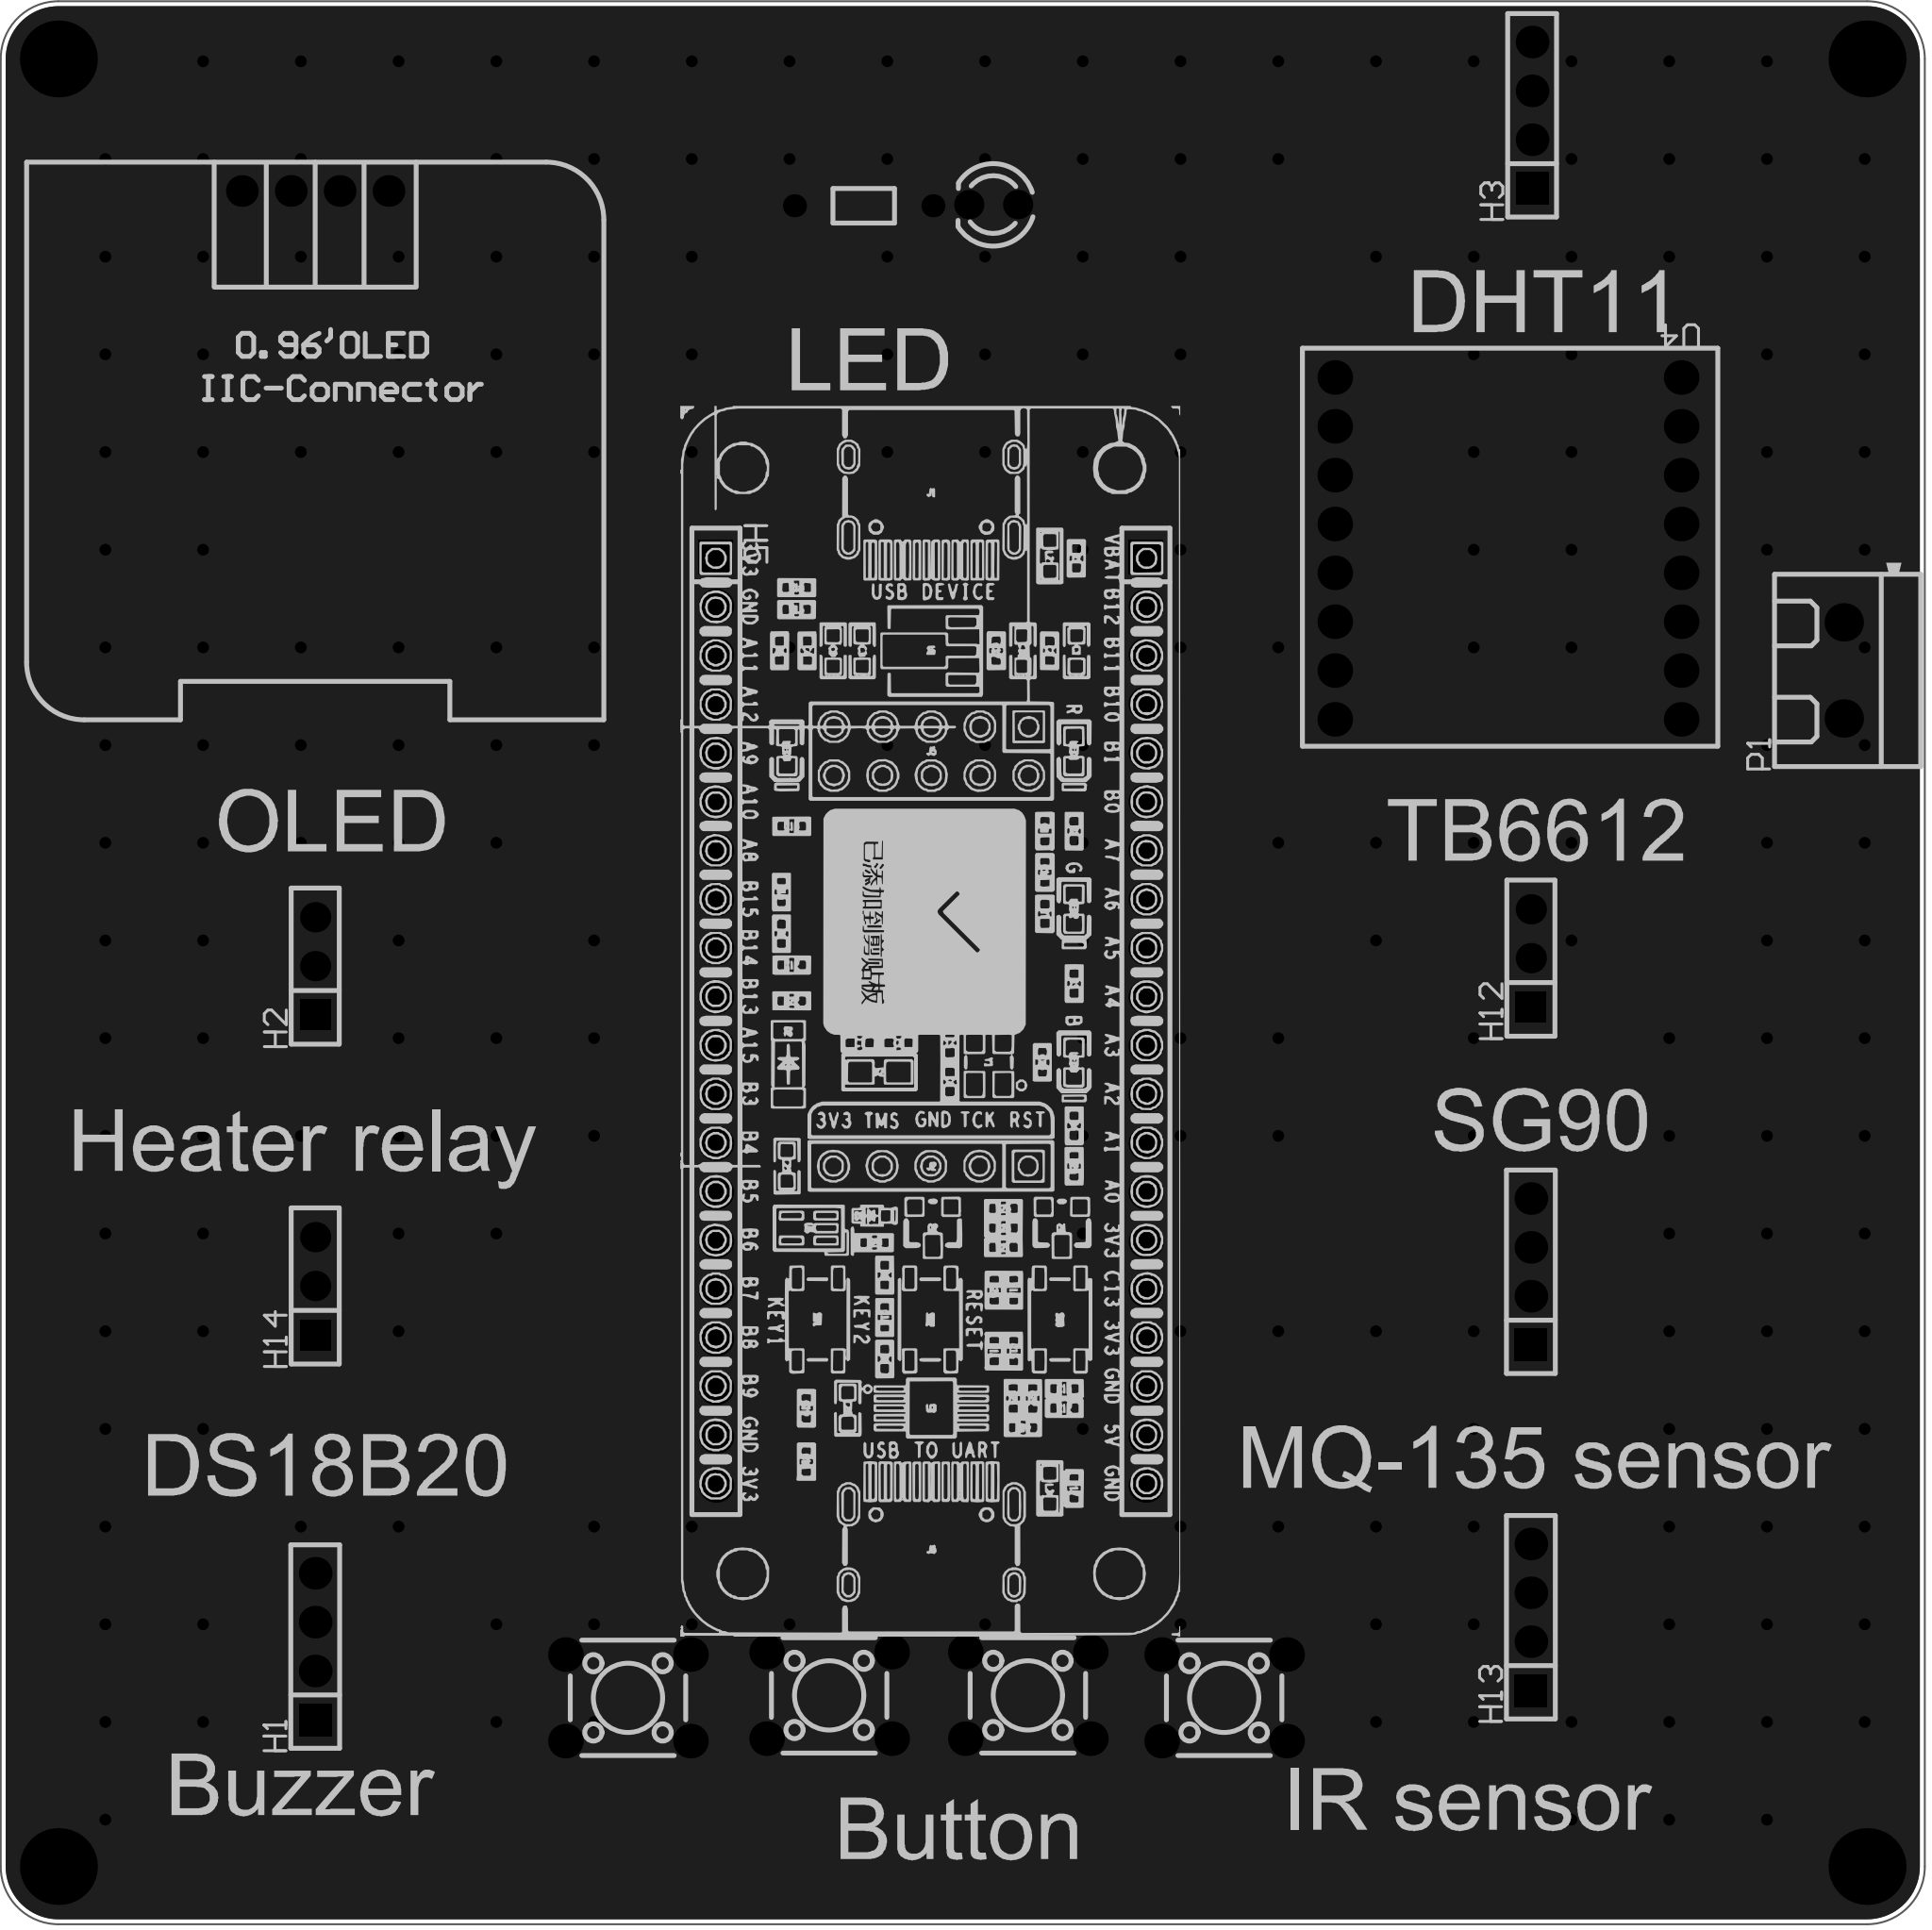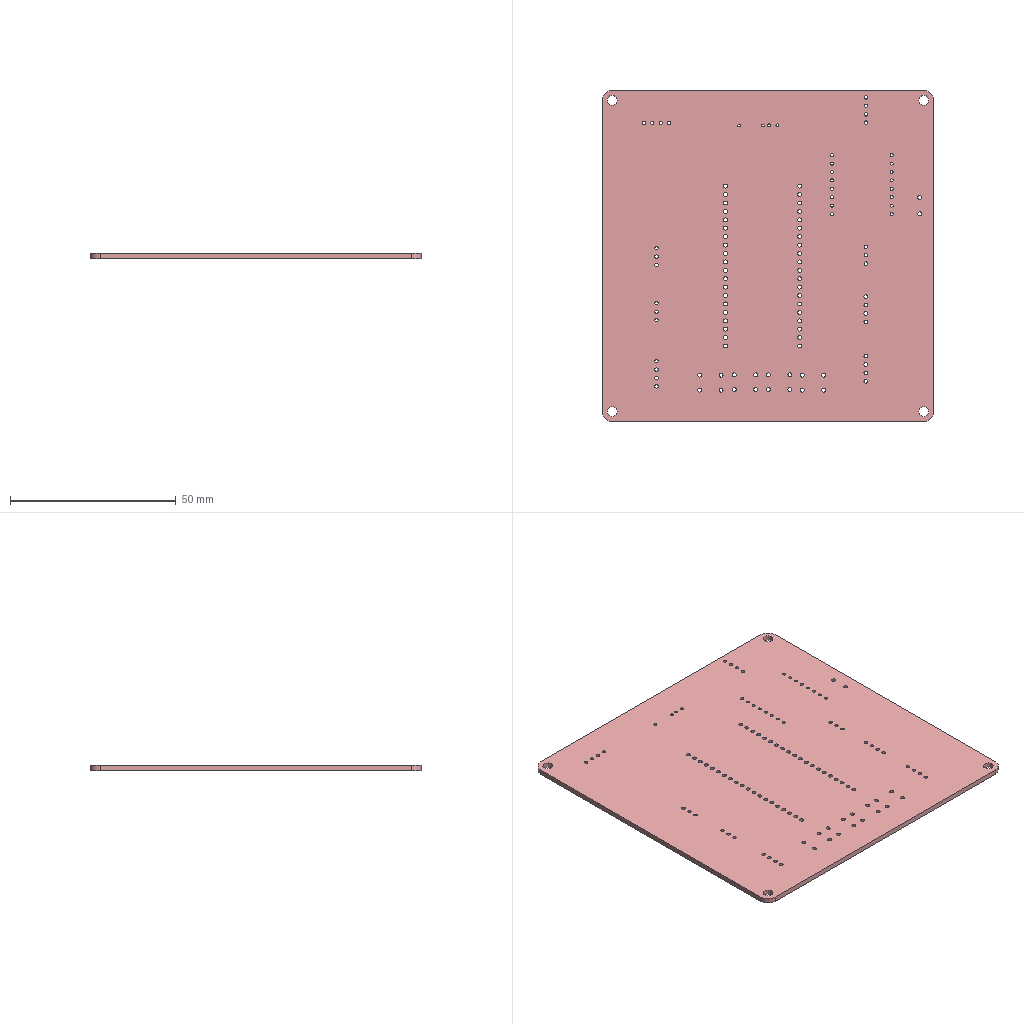Circuit board layout | Altium Designer | box 100 x 100 x 1.6 mm
Layer stack:
# Altium Designer layer stack of  (unit mm; dielectric type: 0 none, 1 core, 2 prepreg, 3 surface material)
index,name,kind,layer,copper_thickness_mm,dielectric_type,dielectric_thickness_mm,dielectric_material,dielectric_constant
0,Top Paste Mask Layer,other,,,,,,
1,Top Silkscreen Layer,other,,,,,,
2,Top Solder Mask Layer,dielectric,,,3,0.01,,3.3
3,Top Layer,copper,Top Layer,0.035,,,,
4,Dielectric1,dielectric,,,3,1.51,FR4,4.5
5,Bottom Layer,copper,Bottom Layer,0.035,,,,
6,Bottom Solder Mask Layer,dielectric,,,3,0.01,,3.3
7,Bottom Silkscreen Layer,other,,,,,,
8,Bottom Paste Mask Layer,other,,,,,,
# drill layer pairs: low layer,high layer
drill_pair,Top Layer,Bottom Layer
Part placement:
Designator,Comment,Layer,Footprint,Center-X(mm),Center-Y(mm),Rotation
SW1,,TopLayer,SW-TH_4P-L6.0-W6.0-P4.50-LS6.5,154.936,92.71,180
SW2,,TopLayer,SW-TH_4P-L6.0-W6.0-P4.50-LS6.5,134.407,92.837,180
SW3,,TopLayer,SW-TH_4P-L6.0-W6.0-P4.50-LS6.5,144.735,92.837,180
SW4,,TopLayer,SW-TH_4P-L6.0-W6.0-P4.50-LS6.5,123.952,92.71,180
H4,,TopLayer,HDR-TH_4P-P2.54-V-F,170.879,114.866,90
H6,,TopLayer,HDR-TH_20P-P2.54-V-F,150.869,127.888,270
LED1,,TopLayer,LED_TH-3mm,142.935,170.363,180
R1,220Ω,TopLayer,Res_1/8W,136.204,170.301,180
H2,,TopLayer,HDR-TH_3P-P2.54-V-F,107.696,130.762,90
OLED1,,TopLayer,0.96OLED_4P,107.696,171.069,0
H12,,TopLayer,HDR-TH_3P-P2.54-V-F,170.879,131.176,90
H13,,TopLayer,HDR-TH_4P-P2.54-V-F,170.879,96.902,90
H14,,TopLayer,HDR-TH_3P-P2.54-V-F,107.696,114.128,90
P1,KF301-2P terminal block,TopLayer,CONN-TH_XY301V-A-5.0-2P,187.141,146.139,90
U4,,TopLayer,tb6612,169.689,152.482,180
H1,,TopLayer,HDR-TH_4P-P2.54-V-F,107.696,95.377,90
H3,,TopLayer,HDR-TH_4P-P2.54-V-F,170.942,175.006,90
H5,,TopLayer,HDR-TH_20P-P2.54-V-F,128.524,127.889,270
Pad and via stacks:
# Altium Designer via and pad stacks of  (unit mm). Each distinct definition once, with the count of objects using it.
# via: kind,start_layer,end_layer,hole_mm,diameter_mm,mode(0 simple;1 top-mid-bottom;2 full stack),diameter_per_layer,count,example_net
# pad: kind,layer,hole_mm,hole_type(0 round;1 square;2 slot),plating,top_size,top_shape(1 round;2 rect;3 octagon;9 rounded rect),mid_size,bottom_size,mode,footprint,size_per_layer,count,example
pad,Multi-Layer,3,0,plated,4x4,1,4x4,4x4,0,,,4,1
pad,Multi-Layer,1.2,0,plated,1.8x1.8,1,1.8x1.8,1.8x1.8,0,SW-TH_4P-L6.0-W6.0-P4.50-LS6.5,,16,SW1.1
pad,Multi-Layer,1.1,0,plated,1.7x1.7,2,1.7x1.7,1.7x1.7,0,HDR-TH_4P-P2.54-V-F,,4,H4.1
pad,Multi-Layer,1.1,0,plated,1.7x1.7,1,1.7x1.7,1.7x1.7,0,HDR-TH_4P-P2.54-V-F,,12,H4.2
pad,Multi-Layer,1.2,0,plated,1.8x1.8,2,1.8x1.8,1.8x1.8,0,HDR-TH_20P-P2.54-V-F,,2,H6.1
pad,Multi-Layer,1.2,0,plated,1.8x1.8,1,1.8x1.8,1.8x1.8,0,HDR-TH_20P-P2.54-V-F,,38,H6.2
pad,Multi-Layer,0.9144,0,plated,1.524x1.524,1,1.524x1.524,1.524x1.524,0,LED_TH-3mm,,2,LED1.1
pad,Multi-Layer,0.8001,0,plated,1.199x1.199,1,1.199x1.199,1.199x1.199,0,Res_1/8W,,2,R1.1
pad,Multi-Layer,1.02,0,plated,1.575x1.575,1,1.575x1.575,1.575x1.575,0,HDR-TH_3P-P2.54-V-F,,6,H2.3
pad,Multi-Layer,1.02,0,plated,1.575x1.575,2,1.575x1.575,1.575x1.575,0,HDR-TH_3P-P2.54-V-F,,3,H2.1
pad,Multi-Layer,1,0,plated,1.65x1.65,1,1.65x1.65,1.65x1.65,0,0.96OLED_4P,,4,OLED1.4
pad,Multi-Layer,1.2,0,plated,2x2,1,2x2,2x2,0,CONN-TH_XY301V-A-5.0-2P,,2,P1.1
pad,Multi-Layer,0.9,0,plated,1.8x1.8,1,1.8x1.8,1.8x1.8,0,tb6612,,16,U4.1
via,Top Layer,Bottom Layer,0.3048,0.61,0,,222,GND
Copper pours:
name,layer,net,type(0 solid;1 hatched;2 none)
Bottom Layer-GND,Bottom Layer,GND,0
Top Layer-GND,Top Layer,GND,0
Design rules, without the lines most boards share:
# Altium Designer design rules of  (exported by Altium Designer, unit mm)
# columns: name | kind | enabled | priority | scope1 | scope2 | descriptor | typed fields (field=value)
Copper_copperRegion_copperThickness1oz | 0 | disabled | 4 | All | All | Clearance Constraint (Gap=5.984mil) (Disabled)(All),(All) | gap=0.152
Copper_copperRegion_copperThickness1oz_1 | 63 | disabled | 4 | All | All | Board Clearance Constraint (Gap=0mil) (Disabled)(All) |
Copper_copperRegion_Copper_copperRegion | 0 | disabled | 5 | All | All | Clearance Constraint (Gap=5.984mil) (Disabled)(All),(All) | gap=0.152
Copper_copperRegion_Copper_copperRegion_1 | 63 | disabled | 5 | All | All | Board Clearance Constraint (Gap=0mil) (Disabled)(All) |
copperThickness1oz | 0 | enabled | 6 | All | All | Clearance Constraint (Gap=5.984mil) (All),(All) | gap=0.152
copperThickness1oz_1 | 63 | enabled | 6 | All | All | Board Clearance Constraint (Gap=0mil) (All) |
copperRegion_copperThickness1oz | 20 | disabled | 1 | All | All | Polygon Connect Rule(Relief Connect )(Conductor Width=10mil) (Relief Angle=90 Angle) (Entries=4) (Air Gap Width=10mil) (Disabled)(All),(All) | connect_style(0=relief,1=direct,2=none)=0 relief_conductor_width=0.254 relief_entries=4
copperRegion_Copper_copperRegion | 20 | disabled | 2 | All | All | Polygon Connect Rule(Relief Connect )(Conductor Width=10mil) (Relief Angle=90 Angle) (Entries=4) (Air Gap Width=10mil) (Disabled)(All),(All) | connect_style(0=relief,1=direct,2=none)=0 relief_conductor_width=0.254 relief_entries=4
copperRegion | 20 | enabled | 3 | All | All | Polygon Connect Rule(Relief Connect )(Conductor Width=10mil) (Relief Angle=90 Angle) (Entries=4) (Air Gap Width=10mil) (All),(All) | connect_style(0=relief,1=direct,2=none)=0 relief_conductor_width=0.254 relief_entries=4